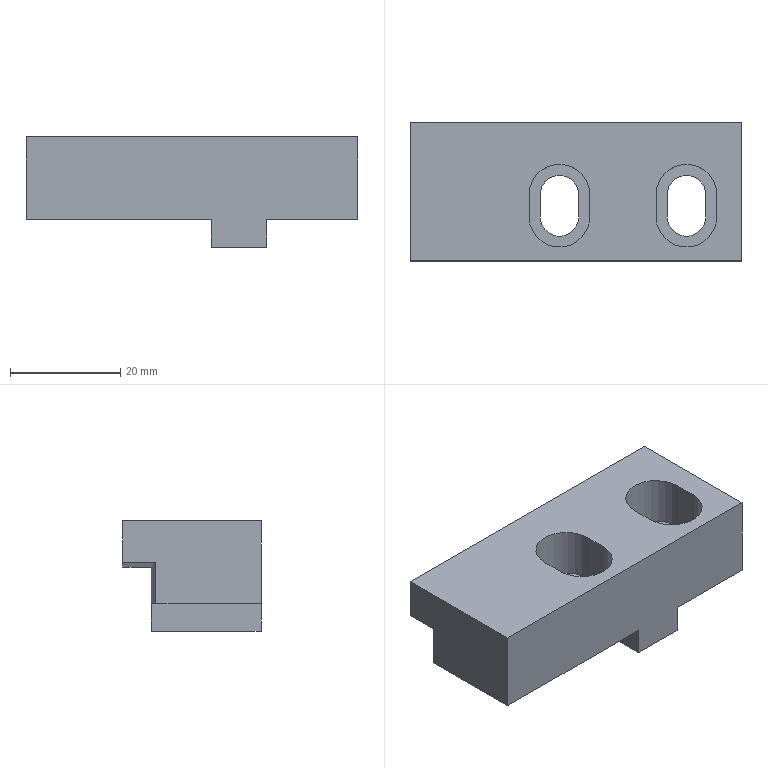Part | NX | features 1605340631 2 | 1 solid | 34 faces | box 60 x 25 x 20 mm | volume 18121 mm3 | plane 26 | cylinder 8 | commonest cylinder face diameters 7 x4 11 x4
STEP:
#1=CARTESIAN_POINT('',(576.,-115.2,-1.5));
#2=VERTEX_POINT('',#1);
#3=CARTESIAN_POINT('',(576.,-95.3,-1.5));
#4=VERTEX_POINT('',#3);
#5=CARTESIAN_POINT('',(576.,-50.,-1.5));
#6=DIRECTION('',(0.,-1.,0.));
#7=VECTOR('',#6,1000.);
#8=LINE('',#5,#7);
#9=EDGE_CURVE('',#2,#4,#8,.F.);
#10=ORIENTED_EDGE('',*,*,#9,.T.);
#11=CARTESIAN_POINT('',(587.5,-95.3,-1.5));
#12=VERTEX_POINT('',#11);
#13=CARTESIAN_POINT('',(560.128,-95.3,-1.5));
#14=DIRECTION('',(-1.,0.,0.));
#15=VECTOR('',#14,1000.);
#16=LINE('',#13,#15);
#17=EDGE_CURVE('',#12,#4,#16,.T.);
#18=ORIENTED_EDGE('',*,*,#17,.F.);
#19=CARTESIAN_POINT('',(592.5,-96.182,-1.5));
#20=VERTEX_POINT('',#19);
#21=CARTESIAN_POINT('',(592.5,-96.182,-1.5));
#22=DIRECTION('',(0.9848,-0.1736,0.));
#23=VECTOR('',#22,1000.);
#24=LINE('',#21,#23);
#25=EDGE_CURVE('',#20,#12,#24,.F.);
#26=ORIENTED_EDGE('',*,*,#25,.F.);
#27=CARTESIAN_POINT('',(592.5,-115.2,-1.5));
#28=VERTEX_POINT('',#27);
#29=CARTESIAN_POINT('',(592.5,-90.2,-1.5));
#30=DIRECTION('',(0.,1.,0.));
#31=VECTOR('',#30,1000.);
#32=LINE('',#29,#31);
#33=EDGE_CURVE('',#28,#20,#32,.T.);
#34=ORIENTED_EDGE('',*,*,#33,.F.);
#35=CARTESIAN_POINT('',(572.,-115.2,-1.5));
#36=DIRECTION('',(1.,0.,0.));
#37=VECTOR('',#36,1000.);
#38=LINE('',#35,#37);
#39=EDGE_CURVE('',#2,#28,#38,.T.);
#40=ORIENTED_EDGE('',*,*,#39,.F.);
#41=EDGE_LOOP('',(#10,#18,#26,#34,#40));
#42=FACE_BOUND('',#41,.T.);
#43=CARTESIAN_POINT('',(579.,-103.2,-1.5));
#44=VERTEX_POINT('',#43);
#45=CARTESIAN_POINT('',(586.,-103.2,-1.5));
#46=VERTEX_POINT('',#45);
#47=CARTESIAN_POINT('',(582.5,-103.2,-1.5));
#48=DIRECTION('',(0.,0.,-1.));
#49=DIRECTION('',(-1.,0.,0.));
#50=AXIS2_PLACEMENT_3D('',#47,#48,#49);
#51=CIRCLE('',#50,3.5);
#52=EDGE_CURVE('',#44,#46,#51,.T.);
#53=ORIENTED_EDGE('',*,*,#52,.F.);
#54=CARTESIAN_POINT('',(579.,-107.2,-1.5));
#55=VERTEX_POINT('',#54);
#56=CARTESIAN_POINT('',(579.,-50.,-1.5));
#57=DIRECTION('',(0.,1.,0.));
#58=VECTOR('',#57,1000.);
#59=LINE('',#56,#58);
#60=EDGE_CURVE('',#44,#55,#59,.F.);
#61=ORIENTED_EDGE('',*,*,#60,.T.);
#62=CARTESIAN_POINT('',(586.,-107.2,-1.5));
#63=VERTEX_POINT('',#62);
#64=CARTESIAN_POINT('',(582.5,-107.2,-1.5));
#65=DIRECTION('',(0.,0.,-1.));
#66=DIRECTION('',(-1.,0.,0.));
#67=AXIS2_PLACEMENT_3D('',#64,#65,#66);
#68=CIRCLE('',#67,3.5);
#69=EDGE_CURVE('',#63,#55,#68,.T.);
#70=ORIENTED_EDGE('',*,*,#69,.F.);
#71=CARTESIAN_POINT('',(586.,-50.,-1.5));
#72=DIRECTION('',(0.,-1.,0.));
#73=VECTOR('',#72,1000.);
#74=LINE('',#71,#73);
#75=EDGE_CURVE('',#63,#46,#74,.F.);
#76=ORIENTED_EDGE('',*,*,#75,.T.);
#77=EDGE_LOOP('',(#53,#61,#70,#76));
#78=FACE_BOUND('',#77,.T.);
#79=CARTESIAN_POINT('',(562.5,-50.,-1.5));
#80=DIRECTION('',(0.,0.,-1.));
#81=DIRECTION('',(-1.,0.,0.));
#82=AXIS2_PLACEMENT_3D('',#79,#80,#81);
#83=PLANE('',#82);
#84=ADVANCED_FACE('',(#42,#78),#83,.T.);
#85=ORIENTED_EDGE('',*,*,#75,.F.);
#86=CARTESIAN_POINT('',(586.,-107.2,4.5));
#87=VERTEX_POINT('',#86);
#88=CARTESIAN_POINT('',(586.,-107.2,1.5));
#89=DIRECTION('',(0.,0.,-1.));
#90=VECTOR('',#89,1000.);
#91=LINE('',#88,#90);
#92=EDGE_CURVE('',#87,#63,#91,.T.);
#93=ORIENTED_EDGE('',*,*,#92,.F.);
#94=CARTESIAN_POINT('',(586.,-103.2,4.5));
#95=VERTEX_POINT('',#94);
#96=CARTESIAN_POINT('',(586.,-105.782,4.5));
#97=DIRECTION('',(0.,-1.,0.));
#98=VECTOR('',#97,1000.);
#99=LINE('',#96,#98);
#100=EDGE_CURVE('',#95,#87,#99,.T.);
#101=ORIENTED_EDGE('',*,*,#100,.F.);
#102=CARTESIAN_POINT('',(586.,-103.2,1.5));
#103=DIRECTION('',(0.,0.,-1.));
#104=VECTOR('',#103,1000.);
#105=LINE('',#102,#104);
#106=EDGE_CURVE('',#46,#95,#105,.F.);
#107=ORIENTED_EDGE('',*,*,#106,.F.);
#108=EDGE_LOOP('',(#85,#93,#101,#107));
#109=FACE_BOUND('',#108,.T.);
#110=CARTESIAN_POINT('',(586.,-105.782,13.5));
#111=DIRECTION('',(1.,0.,0.));
#112=DIRECTION('',(0.,0.,1.));
#113=AXIS2_PLACEMENT_3D('',#110,#111,#112);
#114=PLANE('',#113);
#115=ADVANCED_FACE('',(#109),#114,.F.);
#116=CARTESIAN_POINT('',(588.,-103.2,13.5));
#117=VERTEX_POINT('',#116);
#118=CARTESIAN_POINT('',(577.,-103.2,13.5));
#119=VERTEX_POINT('',#118);
#120=CARTESIAN_POINT('',(582.5,-103.2,13.5));
#121=DIRECTION('',(0.,0.,1.));
#122=DIRECTION('',(1.,0.,0.));
#123=AXIS2_PLACEMENT_3D('',#120,#121,#122);
#124=CIRCLE('',#123,5.5);
#125=EDGE_CURVE('',#117,#119,#124,.T.);
#126=ORIENTED_EDGE('',*,*,#125,.T.);
#127=CARTESIAN_POINT('',(577.,-103.2,4.5));
#128=VERTEX_POINT('',#127);
#129=CARTESIAN_POINT('',(577.,-103.2,9.));
#130=DIRECTION('',(0.,0.,-1.));
#131=VECTOR('',#130,1000.);
#132=LINE('',#129,#131);
#133=EDGE_CURVE('',#119,#128,#132,.T.);
#134=ORIENTED_EDGE('',*,*,#133,.T.);
#135=CARTESIAN_POINT('',(588.,-103.2,4.5));
#136=VERTEX_POINT('',#135);
#137=CARTESIAN_POINT('',(582.5,-103.2,4.5));
#138=DIRECTION('',(0.,0.,-1.));
#139=DIRECTION('',(-1.,0.,0.));
#140=AXIS2_PLACEMENT_3D('',#137,#138,#139);
#141=CIRCLE('',#140,5.5);
#142=EDGE_CURVE('',#136,#128,#141,.F.);
#143=ORIENTED_EDGE('',*,*,#142,.F.);
#144=CARTESIAN_POINT('',(588.,-103.2,9.));
#145=DIRECTION('',(0.,0.,-1.));
#146=VECTOR('',#145,1000.);
#147=LINE('',#144,#146);
#148=EDGE_CURVE('',#136,#117,#147,.F.);
#149=ORIENTED_EDGE('',*,*,#148,.T.);
#150=EDGE_LOOP('',(#126,#134,#143,#149));
#151=FACE_BOUND('',#150,.T.);
#152=CARTESIAN_POINT('',(582.5,-103.2,13.5));
#153=DIRECTION('',(0.,0.,-1.));
#154=DIRECTION('',(-1.,0.,0.));
#155=AXIS2_PLACEMENT_3D('',#152,#153,#154);
#156=CYLINDRICAL_SURFACE('',#155,5.5);
#157=ADVANCED_FACE('',(#151),#156,.F.);
#158=CARTESIAN_POINT('',(588.,-107.2,4.5));
#159=VERTEX_POINT('',#158);
#160=CARTESIAN_POINT('',(577.,-107.2,4.5));
#161=VERTEX_POINT('',#160);
#162=CARTESIAN_POINT('',(582.5,-107.2,4.5));
#163=DIRECTION('',(0.,0.,-1.));
#164=DIRECTION('',(-1.,0.,0.));
#165=AXIS2_PLACEMENT_3D('',#162,#163,#164);
#166=CIRCLE('',#165,5.5);
#167=EDGE_CURVE('',#159,#161,#166,.T.);
#168=ORIENTED_EDGE('',*,*,#167,.T.);
#169=CARTESIAN_POINT('',(577.,-107.2,13.5));
#170=VERTEX_POINT('',#169);
#171=CARTESIAN_POINT('',(577.,-107.2,9.));
#172=DIRECTION('',(0.,0.,-1.));
#173=VECTOR('',#172,1000.);
#174=LINE('',#171,#173);
#175=EDGE_CURVE('',#161,#170,#174,.F.);
#176=ORIENTED_EDGE('',*,*,#175,.T.);
#177=CARTESIAN_POINT('',(588.,-107.2,13.5));
#178=VERTEX_POINT('',#177);
#179=CARTESIAN_POINT('',(582.5,-107.2,13.5));
#180=DIRECTION('',(0.,0.,1.));
#181=DIRECTION('',(1.,0.,0.));
#182=AXIS2_PLACEMENT_3D('',#179,#180,#181);
#183=CIRCLE('',#182,5.5);
#184=EDGE_CURVE('',#170,#178,#183,.T.);
#185=ORIENTED_EDGE('',*,*,#184,.T.);
#186=CARTESIAN_POINT('',(588.,-107.2,9.));
#187=DIRECTION('',(0.,0.,-1.));
#188=VECTOR('',#187,1000.);
#189=LINE('',#186,#188);
#190=EDGE_CURVE('',#178,#159,#189,.T.);
#191=ORIENTED_EDGE('',*,*,#190,.T.);
#192=EDGE_LOOP('',(#168,#176,#185,#191));
#193=FACE_BOUND('',#192,.T.);
#194=CARTESIAN_POINT('',(582.5,-107.2,13.5));
#195=DIRECTION('',(0.,0.,-1.));
#196=DIRECTION('',(-1.,0.,0.));
#197=AXIS2_PLACEMENT_3D('',#194,#195,#196);
#198=CYLINDRICAL_SURFACE('',#197,5.5);
#199=ADVANCED_FACE('',(#193),#198,.F.);
#200=CARTESIAN_POINT('',(579.,-107.2,4.5));
#201=VERTEX_POINT('',#200);
#202=CARTESIAN_POINT('',(582.5,-107.2,4.5));
#203=DIRECTION('',(0.,0.,1.));
#204=DIRECTION('',(1.,0.,0.));
#205=AXIS2_PLACEMENT_3D('',#202,#203,#204);
#206=CIRCLE('',#205,3.5);
#207=EDGE_CURVE('',#87,#201,#206,.F.);
#208=ORIENTED_EDGE('',*,*,#207,.T.);
#209=CARTESIAN_POINT('',(579.,-103.2,4.5));
#210=VERTEX_POINT('',#209);
#211=CARTESIAN_POINT('',(579.,-105.782,4.5));
#212=DIRECTION('',(0.,1.,0.));
#213=VECTOR('',#212,1000.);
#214=LINE('',#211,#213);
#215=EDGE_CURVE('',#201,#210,#214,.T.);
#216=ORIENTED_EDGE('',*,*,#215,.T.);
#217=CARTESIAN_POINT('',(582.5,-103.2,4.5));
#218=DIRECTION('',(0.,0.,1.));
#219=DIRECTION('',(1.,0.,0.));
#220=AXIS2_PLACEMENT_3D('',#217,#218,#219);
#221=CIRCLE('',#220,3.5);
#222=EDGE_CURVE('',#95,#210,#221,.T.);
#223=ORIENTED_EDGE('',*,*,#222,.F.);
#224=ORIENTED_EDGE('',*,*,#100,.T.);
#225=EDGE_LOOP('',(#208,#216,#223,#224));
#226=FACE_BOUND('',#225,.T.);
#227=ORIENTED_EDGE('',*,*,#167,.F.);
#228=CARTESIAN_POINT('',(588.,-107.2,4.5));
#229=DIRECTION('',(0.,1.,0.));
#230=VECTOR('',#229,1000.);
#231=LINE('',#228,#230);
#232=EDGE_CURVE('',#159,#136,#231,.T.);
#233=ORIENTED_EDGE('',*,*,#232,.T.);
#234=ORIENTED_EDGE('',*,*,#142,.T.);
#235=CARTESIAN_POINT('',(577.,-107.2,4.5));
#236=DIRECTION('',(0.,-1.,0.));
#237=VECTOR('',#236,1000.);
#238=LINE('',#235,#237);
#239=EDGE_CURVE('',#128,#161,#238,.T.);
#240=ORIENTED_EDGE('',*,*,#239,.T.);
#241=EDGE_LOOP('',(#227,#233,#234,#240));
#242=FACE_BOUND('',#241,.T.);
#243=CARTESIAN_POINT('',(582.5,-107.2,4.5));
#244=DIRECTION('',(0.,0.,-1.));
#245=DIRECTION('',(1.,0.,0.));
#246=AXIS2_PLACEMENT_3D('',#243,#244,#245);
#247=PLANE('',#246);
#248=ADVANCED_FACE('',(#226,#242),#247,.F.);
#249=ORIENTED_EDGE('',*,*,#232,.F.);
#250=ORIENTED_EDGE('',*,*,#190,.F.);
#251=CARTESIAN_POINT('',(588.,-107.951,13.5));
#252=DIRECTION('',(0.,1.,0.));
#253=VECTOR('',#252,1000.);
#254=LINE('',#251,#253);
#255=EDGE_CURVE('',#117,#178,#254,.F.);
#256=ORIENTED_EDGE('',*,*,#255,.F.);
#257=ORIENTED_EDGE('',*,*,#148,.F.);
#258=EDGE_LOOP('',(#249,#250,#256,#257));
#259=FACE_BOUND('',#258,.T.);
#260=CARTESIAN_POINT('',(588.,-105.836,13.5));
#261=DIRECTION('',(1.,0.,0.));
#262=DIRECTION('',(0.,0.,1.));
#263=AXIS2_PLACEMENT_3D('',#260,#261,#262);
#264=PLANE('',#263);
#265=ADVANCED_FACE('',(#259),#264,.F.);
#266=CARTESIAN_POINT('',(577.,-107.951,13.5));
#267=DIRECTION('',(0.,-1.,0.));
#268=VECTOR('',#267,1000.);
#269=LINE('',#266,#268);
#270=EDGE_CURVE('',#170,#119,#269,.F.);
#271=ORIENTED_EDGE('',*,*,#270,.F.);
#272=ORIENTED_EDGE('',*,*,#175,.F.);
#273=ORIENTED_EDGE('',*,*,#239,.F.);
#274=ORIENTED_EDGE('',*,*,#133,.F.);
#275=EDGE_LOOP('',(#271,#272,#273,#274));
#276=FACE_BOUND('',#275,.T.);
#277=CARTESIAN_POINT('',(577.,-105.836,13.5));
#278=DIRECTION('',(-1.,0.,0.));
#279=DIRECTION('',(0.,0.,-1.));
#280=AXIS2_PLACEMENT_3D('',#277,#278,#279);
#281=PLANE('',#280);
#282=ADVANCED_FACE('',(#276),#281,.F.);
#283=ORIENTED_EDGE('',*,*,#215,.F.);
#284=CARTESIAN_POINT('',(579.,-107.2,1.5));
#285=DIRECTION('',(0.,0.,-1.));
#286=VECTOR('',#285,1000.);
#287=LINE('',#284,#286);
#288=EDGE_CURVE('',#55,#201,#287,.F.);
#289=ORIENTED_EDGE('',*,*,#288,.F.);
#290=ORIENTED_EDGE('',*,*,#60,.F.);
#291=CARTESIAN_POINT('',(579.,-103.2,1.5));
#292=DIRECTION('',(0.,0.,-1.));
#293=VECTOR('',#292,1000.);
#294=LINE('',#291,#293);
#295=EDGE_CURVE('',#210,#44,#294,.T.);
#296=ORIENTED_EDGE('',*,*,#295,.F.);
#297=EDGE_LOOP('',(#283,#289,#290,#296));
#298=FACE_BOUND('',#297,.T.);
#299=CARTESIAN_POINT('',(579.,-105.782,13.5));
#300=DIRECTION('',(-1.,0.,0.));
#301=DIRECTION('',(0.,0.,-1.));
#302=AXIS2_PLACEMENT_3D('',#299,#300,#301);
#303=PLANE('',#302);
#304=ADVANCED_FACE('',(#298),#303,.F.);
#305=ORIENTED_EDGE('',*,*,#69,.T.);
#306=ORIENTED_EDGE('',*,*,#288,.T.);
#307=ORIENTED_EDGE('',*,*,#207,.F.);
#308=ORIENTED_EDGE('',*,*,#92,.T.);
#309=EDGE_LOOP('',(#305,#306,#307,#308));
#310=FACE_BOUND('',#309,.T.);
#311=CARTESIAN_POINT('',(582.5,-107.2,13.5));
#312=DIRECTION('',(0.,0.,-1.));
#313=DIRECTION('',(-1.,0.,0.));
#314=AXIS2_PLACEMENT_3D('',#311,#312,#313);
#315=CYLINDRICAL_SURFACE('',#314,3.5);
#316=ADVANCED_FACE('',(#310),#315,.F.);
#317=ORIENTED_EDGE('',*,*,#222,.T.);
#318=ORIENTED_EDGE('',*,*,#295,.T.);
#319=ORIENTED_EDGE('',*,*,#52,.T.);
#320=ORIENTED_EDGE('',*,*,#106,.T.);
#321=EDGE_LOOP('',(#317,#318,#319,#320));
#322=FACE_BOUND('',#321,.T.);
#323=CARTESIAN_POINT('',(582.5,-103.2,13.5));
#324=DIRECTION('',(0.,0.,-1.));
#325=DIRECTION('',(-1.,0.,0.));
#326=AXIS2_PLACEMENT_3D('',#323,#324,#325);
#327=CYLINDRICAL_SURFACE('',#326,3.5);
#328=ADVANCED_FACE('',(#322),#327,.F.);
#329=CARTESIAN_POINT('',(563.,-107.2,4.5));
#330=VERTEX_POINT('',#329);
#331=CARTESIAN_POINT('',(556.,-107.2,4.5));
#332=VERTEX_POINT('',#331);
#333=CARTESIAN_POINT('',(559.5,-107.2,4.5));
#334=DIRECTION('',(0.,0.,-1.));
#335=DIRECTION('',(-1.,0.,0.));
#336=AXIS2_PLACEMENT_3D('',#333,#334,#335);
#337=CIRCLE('',#336,3.5);
#338=EDGE_CURVE('',#330,#332,#337,.T.);
#339=ORIENTED_EDGE('',*,*,#338,.T.);
#340=CARTESIAN_POINT('',(556.,-103.2,4.5));
#341=VERTEX_POINT('',#340);
#342=CARTESIAN_POINT('',(556.,-105.782,4.5));
#343=DIRECTION('',(0.,-1.,0.));
#344=VECTOR('',#343,1000.);
#345=LINE('',#342,#344);
#346=EDGE_CURVE('',#332,#341,#345,.F.);
#347=ORIENTED_EDGE('',*,*,#346,.T.);
#348=CARTESIAN_POINT('',(563.,-103.2,4.5));
#349=VERTEX_POINT('',#348);
#350=CARTESIAN_POINT('',(559.5,-103.2,4.5));
#351=DIRECTION('',(0.,0.,-1.));
#352=DIRECTION('',(-1.,0.,0.));
#353=AXIS2_PLACEMENT_3D('',#350,#351,#352);
#354=CIRCLE('',#353,3.5);
#355=EDGE_CURVE('',#349,#341,#354,.F.);
#356=ORIENTED_EDGE('',*,*,#355,.F.);
#357=CARTESIAN_POINT('',(563.,-105.782,4.5));
#358=DIRECTION('',(0.,1.,0.));
#359=VECTOR('',#358,1000.);
#360=LINE('',#357,#359);
#361=EDGE_CURVE('',#349,#330,#360,.F.);
#362=ORIENTED_EDGE('',*,*,#361,.T.);
#363=EDGE_LOOP('',(#339,#347,#356,#362));
#364=FACE_BOUND('',#363,.T.);
#365=CARTESIAN_POINT('',(565.,-107.2,4.5));
#366=VERTEX_POINT('',#365);
#367=CARTESIAN_POINT('',(554.,-107.2,4.5));
#368=VERTEX_POINT('',#367);
#369=CARTESIAN_POINT('',(559.5,-107.2,4.5));
#370=DIRECTION('',(0.,0.,1.));
#371=DIRECTION('',(1.,0.,0.));
#372=AXIS2_PLACEMENT_3D('',#369,#370,#371);
#373=CIRCLE('',#372,5.5);
#374=EDGE_CURVE('',#366,#368,#373,.F.);
#375=ORIENTED_EDGE('',*,*,#374,.F.);
#376=CARTESIAN_POINT('',(565.,-103.2,4.5));
#377=VERTEX_POINT('',#376);
#378=CARTESIAN_POINT('',(565.,-107.2,4.5));
#379=DIRECTION('',(0.,-1.,0.));
#380=VECTOR('',#379,1000.);
#381=LINE('',#378,#380);
#382=EDGE_CURVE('',#366,#377,#381,.F.);
#383=ORIENTED_EDGE('',*,*,#382,.T.);
#384=CARTESIAN_POINT('',(554.,-103.2,4.5));
#385=VERTEX_POINT('',#384);
#386=CARTESIAN_POINT('',(559.5,-103.2,4.5));
#387=DIRECTION('',(0.,0.,1.));
#388=DIRECTION('',(1.,0.,0.));
#389=AXIS2_PLACEMENT_3D('',#386,#387,#388);
#390=CIRCLE('',#389,5.5);
#391=EDGE_CURVE('',#377,#385,#390,.T.);
#392=ORIENTED_EDGE('',*,*,#391,.T.);
#393=CARTESIAN_POINT('',(554.,-107.2,4.5));
#394=DIRECTION('',(0.,1.,0.));
#395=VECTOR('',#394,1000.);
#396=LINE('',#393,#395);
#397=EDGE_CURVE('',#385,#368,#396,.F.);
#398=ORIENTED_EDGE('',*,*,#397,.T.);
#399=EDGE_LOOP('',(#375,#383,#392,#398));
#400=FACE_BOUND('',#399,.T.);
#401=CARTESIAN_POINT('',(542.5,-107.2,4.5));
#402=DIRECTION('',(0.,0.,-1.));
#403=DIRECTION('',(-1.,0.,0.));
#404=AXIS2_PLACEMENT_3D('',#401,#402,#403);
#405=PLANE('',#404);
#406=ADVANCED_FACE('',(#364,#400),#405,.F.);
#407=CARTESIAN_POINT('',(537.5,-95.3,5.1));
#408=VERTEX_POINT('',#407);
#409=CARTESIAN_POINT('',(532.5,-96.182,5.982));
#410=VERTEX_POINT('',#409);
#411=CARTESIAN_POINT('',(535.027,-95.736,5.536));
#412=DIRECTION('',(-0.9703,-0.1711,0.1711));
#413=VECTOR('',#412,1000.);
#414=LINE('',#411,#413);
#415=EDGE_CURVE('',#408,#410,#414,.T.);
#416=ORIENTED_EDGE('',*,*,#415,.T.);
#417=CARTESIAN_POINT('',(532.5,-90.2,5.982));
#418=VERTEX_POINT('',#417);
#419=CARTESIAN_POINT('',(532.5,-95.3,5.982));
#420=DIRECTION('',(0.,-1.,0.));
#421=VECTOR('',#420,1000.);
#422=LINE('',#419,#421);
#423=EDGE_CURVE('',#418,#410,#422,.T.);
#424=ORIENTED_EDGE('',*,*,#423,.F.);
#425=CARTESIAN_POINT('',(537.5,-90.2,5.1));
#426=VERTEX_POINT('',#425);
#427=CARTESIAN_POINT('',(543.856,-90.2,3.979));
#428=DIRECTION('',(-0.9848,0.,0.1736));
#429=VECTOR('',#428,1000.);
#430=LINE('',#427,#429);
#431=EDGE_CURVE('',#426,#418,#430,.T.);
#432=ORIENTED_EDGE('',*,*,#431,.F.);
#433=CARTESIAN_POINT('',(537.5,-92.2,5.1));
#434=DIRECTION('',(0.,1.,0.));
#435=VECTOR('',#434,1000.);
#436=LINE('',#433,#435);
#437=EDGE_CURVE('',#408,#426,#436,.T.);
#438=ORIENTED_EDGE('',*,*,#437,.F.);
#439=EDGE_LOOP('',(#416,#424,#432,#438));
#440=FACE_BOUND('',#439,.T.);
#441=CARTESIAN_POINT('',(537.5,-110.2,5.1));
#442=DIRECTION('',(-0.1736,0.,-0.9848));
#443=DIRECTION('',(0.,-1.,0.));
#444=AXIS2_PLACEMENT_3D('',#441,#442,#443);
#445=PLANE('',#444);
#446=ADVANCED_FACE('',(#440),#445,.T.);
#447=CARTESIAN_POINT('',(587.5,-90.2,5.1));
#448=VERTEX_POINT('',#447);
#449=CARTESIAN_POINT('',(552.,-90.2,5.1));
#450=DIRECTION('',(1.,0.,0.));
#451=VECTOR('',#450,1000.);
#452=LINE('',#449,#451);
#453=EDGE_CURVE('',#426,#448,#452,.T.);
#454=ORIENTED_EDGE('',*,*,#453,.T.);
#455=CARTESIAN_POINT('',(587.5,-95.3,5.1));
#456=VERTEX_POINT('',#455);
#457=CARTESIAN_POINT('',(587.5,-95.3,5.1));
#458=DIRECTION('',(0.,-1.,0.));
#459=VECTOR('',#458,1000.);
#460=LINE('',#457,#459);
#461=EDGE_CURVE('',#448,#456,#460,.T.);
#462=ORIENTED_EDGE('',*,*,#461,.T.);
#463=CARTESIAN_POINT('',(560.128,-95.3,5.1));
#464=DIRECTION('',(1.,0.,0.));
#465=VECTOR('',#464,1000.);
#466=LINE('',#463,#465);
#467=EDGE_CURVE('',#408,#456,#466,.T.);
#468=ORIENTED_EDGE('',*,*,#467,.F.);
#469=ORIENTED_EDGE('',*,*,#437,.T.);
#470=EDGE_LOOP('',(#454,#462,#468,#469));
#471=FACE_BOUND('',#470,.T.);
#472=CARTESIAN_POINT('',(552.,-110.2,5.1));
#473=DIRECTION('',(0.,0.,1.));
#474=DIRECTION('',(1.,0.,0.));
#475=AXIS2_PLACEMENT_3D('',#472,#473,#474);
#476=PLANE('',#475);
#477=ADVANCED_FACE('',(#471),#476,.F.);
#478=CARTESIAN_POINT('',(592.5,-90.2,5.982));
#479=VERTEX_POINT('',#478);
#480=CARTESIAN_POINT('',(561.747,-90.2,0.5591));
#481=DIRECTION('',(-0.9848,0.,-0.1736));
#482=VECTOR('',#481,1000.);
#483=LINE('',#480,#482);
#484=EDGE_CURVE('',#479,#448,#483,.T.);
#485=ORIENTED_EDGE('',*,*,#484,.F.);
#486=CARTESIAN_POINT('',(592.5,-96.182,5.982));
#487=VERTEX_POINT('',#486);
#488=CARTESIAN_POINT('',(592.5,-92.2,5.982));
#489=DIRECTION('',(0.,1.,0.));
#490=VECTOR('',#489,1000.);
#491=LINE('',#488,#490);
#492=EDGE_CURVE('',#487,#479,#491,.T.);
#493=ORIENTED_EDGE('',*,*,#492,.F.);
#494=CARTESIAN_POINT('',(589.973,-95.736,5.536));
#495=DIRECTION('',(-0.9703,0.1711,-0.1711));
#496=VECTOR('',#495,1000.);
#497=LINE('',#494,#496);
#498=EDGE_CURVE('',#487,#456,#497,.T.);
#499=ORIENTED_EDGE('',*,*,#498,.T.);
#500=ORIENTED_EDGE('',*,*,#461,.F.);
#501=EDGE_LOOP('',(#485,#493,#499,#500));
#502=FACE_BOUND('',#501,.T.);
#503=CARTESIAN_POINT('',(587.5,-110.2,5.1));
#504=DIRECTION('',(0.1736,0.,-0.9848));
#505=DIRECTION('',(0.,1.,0.));
#506=AXIS2_PLACEMENT_3D('',#503,#504,#505);
#507=PLANE('',#506);
#508=ADVANCED_FACE('',(#502),#507,.T.);
#509=CARTESIAN_POINT('',(592.5,-96.182,-36.501));
#510=DIRECTION('',(0.,0.,1.));
#511=VECTOR('',#510,1000.);
#512=LINE('',#509,#511);
#513=EDGE_CURVE('',#20,#487,#512,.T.);
#514=ORIENTED_EDGE('',*,*,#513,.F.);
#515=ORIENTED_EDGE('',*,*,#25,.T.);
#516=CARTESIAN_POINT('',(587.5,-95.3,-0.1));
#517=DIRECTION('',(0.,0.,-1.));
#518=VECTOR('',#517,1000.);
#519=LINE('',#516,#518);
#520=EDGE_CURVE('',#456,#12,#519,.T.);
#521=ORIENTED_EDGE('',*,*,#520,.F.);
#522=ORIENTED_EDGE('',*,*,#498,.F.);
#523=EDGE_LOOP('',(#514,#515,#521,#522));
#524=FACE_BOUND('',#523,.T.);
#525=CARTESIAN_POINT('',(592.5,-96.182,-36.501));
#526=DIRECTION('',(-0.1736,-0.9848,0.));
#527=DIRECTION('',(0.,0.,1.));
#528=AXIS2_PLACEMENT_3D('',#525,#526,#527);
#529=PLANE('',#528);
#530=ADVANCED_FACE('',(#524),#529,.F.);
#531=ORIENTED_EDGE('',*,*,#17,.T.);
#532=CARTESIAN_POINT('',(576.,-95.3,-6.5));
#533=VERTEX_POINT('',#532);
#534=CARTESIAN_POINT('',(576.,-95.3,-6.5));
#535=DIRECTION('',(0.,0.,1.));
#536=VECTOR('',#535,1000.);
#537=LINE('',#534,#536);
#538=EDGE_CURVE('',#4,#533,#537,.F.);
#539=ORIENTED_EDGE('',*,*,#538,.T.);
#540=CARTESIAN_POINT('',(566.,-95.3,-6.5));
#541=VERTEX_POINT('',#540);
#542=CARTESIAN_POINT('',(560.128,-95.3,-6.5));
#543=DIRECTION('',(-1.,0.,0.));
#544=VECTOR('',#543,1000.);
#545=LINE('',#542,#544);
#546=EDGE_CURVE('',#541,#533,#545,.F.);
#547=ORIENTED_EDGE('',*,*,#546,.F.);
#548=CARTESIAN_POINT('',(566.,-95.3,-1.5));
#549=VERTEX_POINT('',#548);
#550=CARTESIAN_POINT('',(566.,-95.3,-0.1));
#551=DIRECTION('',(0.,0.,1.));
#552=VECTOR('',#551,1000.);
#553=LINE('',#550,#552);
#554=EDGE_CURVE('',#549,#541,#553,.F.);
#555=ORIENTED_EDGE('',*,*,#554,.F.);
#556=CARTESIAN_POINT('',(537.5,-95.3,-1.5));
#557=VERTEX_POINT('',#556);
#558=CARTESIAN_POINT('',(560.128,-95.3,-1.5));
#559=DIRECTION('',(-1.,0.,0.));
#560=VECTOR('',#559,1000.);
#561=LINE('',#558,#560);
#562=EDGE_CURVE('',#549,#557,#561,.T.);
#563=ORIENTED_EDGE('',*,*,#562,.T.);
#564=CARTESIAN_POINT('',(537.5,-95.3,-0.1));
#565=DIRECTION('',(0.,0.,1.));
#566=VECTOR('',#565,1000.);
#567=LINE('',#564,#566);
#568=EDGE_CURVE('',#557,#408,#567,.T.);
#569=ORIENTED_EDGE('',*,*,#568,.T.);
#570=ORIENTED_EDGE('',*,*,#467,.T.);
#571=ORIENTED_EDGE('',*,*,#520,.T.);
#572=EDGE_LOOP('',(#531,#539,#547,#555,#563,#569,#570,#571));
#573=FACE_BOUND('',#572,.T.);
#574=CARTESIAN_POINT('',(560.128,-95.3,-0.1));
#575=DIRECTION('',(0.,1.,0.));
#576=DIRECTION('',(-1.,0.,0.));
#577=AXIS2_PLACEMENT_3D('',#574,#575,#576);
#578=PLANE('',#577);
#579=ADVANCED_FACE('',(#573),#578,.T.);
#580=ORIENTED_EDGE('',*,*,#568,.F.);
#581=CARTESIAN_POINT('',(532.5,-96.182,-1.5));
#582=VERTEX_POINT('',#581);
#583=CARTESIAN_POINT('',(532.5,-96.182,-1.5));
#584=DIRECTION('',(0.9848,0.1736,0.));
#585=VECTOR('',#584,1000.);
#586=LINE('',#583,#585);
#587=EDGE_CURVE('',#557,#582,#586,.F.);
#588=ORIENTED_EDGE('',*,*,#587,.T.);
#589=CARTESIAN_POINT('',(532.5,-96.182,-36.501));
#590=DIRECTION('',(0.,0.,-1.));
#591=VECTOR('',#590,1000.);
#592=LINE('',#589,#591);
#593=EDGE_CURVE('',#410,#582,#592,.T.);
#594=ORIENTED_EDGE('',*,*,#593,.F.);
#595=ORIENTED_EDGE('',*,*,#415,.F.);
#596=EDGE_LOOP('',(#580,#588,#594,#595));
#597=FACE_BOUND('',#596,.T.);
#598=CARTESIAN_POINT('',(532.5,-96.182,-36.501));
#599=DIRECTION('',(0.1736,-0.9848,0.));
#600=DIRECTION('',(0.,0.,-1.));
#601=AXIS2_PLACEMENT_3D('',#598,#599,#600);
#602=PLANE('',#601);
#603=ADVANCED_FACE('',(#597),#602,.F.);
#604=CARTESIAN_POINT('',(565.,-103.2,13.5));
#605=VERTEX_POINT('',#604);
#606=CARTESIAN_POINT('',(565.,-107.2,13.5));
#607=VERTEX_POINT('',#606);
#608=CARTESIAN_POINT('',(565.,-107.951,13.5));
#609=DIRECTION('',(0.,1.,0.));
#610=VECTOR('',#609,1000.);
#611=LINE('',#608,#610);
#612=EDGE_CURVE('',#605,#607,#611,.F.);
#613=ORIENTED_EDGE('',*,*,#612,.F.);
#614=CARTESIAN_POINT('',(565.,-103.2,9.));
#615=DIRECTION('',(0.,0.,-1.));
#616=VECTOR('',#615,1000.);
#617=LINE('',#614,#616);
#618=EDGE_CURVE('',#377,#605,#617,.F.);
#619=ORIENTED_EDGE('',*,*,#618,.F.);
#620=ORIENTED_EDGE('',*,*,#382,.F.);
#621=CARTESIAN_POINT('',(565.,-107.2,9.));
#622=DIRECTION('',(0.,0.,-1.));
#623=VECTOR('',#622,1000.);
#624=LINE('',#621,#623);
#625=EDGE_CURVE('',#607,#366,#624,.T.);
#626=ORIENTED_EDGE('',*,*,#625,.F.);
#627=EDGE_LOOP('',(#613,#619,#620,#626));
#628=FACE_BOUND('',#627,.T.);
#629=CARTESIAN_POINT('',(565.,-105.836,13.5));
#630=DIRECTION('',(1.,0.,0.));
#631=DIRECTION('',(0.,0.,-1.));
#632=AXIS2_PLACEMENT_3D('',#629,#630,#631);
#633=PLANE('',#632);
#634=ADVANCED_FACE('',(#628),#633,.F.);
#635=CARTESIAN_POINT('',(554.,-103.2,13.5));
#636=VERTEX_POINT('',#635);
#637=CARTESIAN_POINT('',(559.5,-103.2,13.5));
#638=DIRECTION('',(0.,0.,-1.));
#639=DIRECTION('',(1.,0.,0.));
#640=AXIS2_PLACEMENT_3D('',#637,#638,#639);
#641=CIRCLE('',#640,5.5);
#642=EDGE_CURVE('',#636,#605,#641,.T.);
#643=ORIENTED_EDGE('',*,*,#642,.F.);
#644=CARTESIAN_POINT('',(554.,-103.2,9.));
#645=DIRECTION('',(0.,0.,-1.));
#646=VECTOR('',#645,1000.);
#647=LINE('',#644,#646);
#648=EDGE_CURVE('',#636,#385,#647,.T.);
#649=ORIENTED_EDGE('',*,*,#648,.T.);
#650=ORIENTED_EDGE('',*,*,#391,.F.);
#651=ORIENTED_EDGE('',*,*,#618,.T.);
#652=EDGE_LOOP('',(#643,#649,#650,#651));
#653=FACE_BOUND('',#652,.T.);
#654=CARTESIAN_POINT('',(559.5,-103.2,13.5));
#655=DIRECTION('',(0.,0.,-1.));
#656=DIRECTION('',(1.,0.,0.));
#657=AXIS2_PLACEMENT_3D('',#654,#655,#656);
#658=CYLINDRICAL_SURFACE('',#657,5.5);
#659=ADVANCED_FACE('',(#653),#658,.F.);
#660=ORIENTED_EDGE('',*,*,#397,.F.);
#661=ORIENTED_EDGE('',*,*,#648,.F.);
#662=CARTESIAN_POINT('',(554.,-107.2,13.5));
#663=VERTEX_POINT('',#662);
#664=CARTESIAN_POINT('',(554.,-107.951,13.5));
#665=DIRECTION('',(0.,-1.,0.));
#666=VECTOR('',#665,1000.);
#667=LINE('',#664,#666);
#668=EDGE_CURVE('',#663,#636,#667,.F.);
#669=ORIENTED_EDGE('',*,*,#668,.F.);
#670=CARTESIAN_POINT('',(554.,-107.2,9.));
#671=DIRECTION('',(0.,0.,-1.));
#672=VECTOR('',#671,1000.);
#673=LINE('',#670,#672);
#674=EDGE_CURVE('',#368,#663,#673,.F.);
#675=ORIENTED_EDGE('',*,*,#674,.F.);
#676=EDGE_LOOP('',(#660,#661,#669,#675));
#677=FACE_BOUND('',#676,.T.);
#678=CARTESIAN_POINT('',(554.,-105.836,13.5));
#679=DIRECTION('',(-1.,0.,0.));
#680=DIRECTION('',(0.,0.,1.));
#681=AXIS2_PLACEMENT_3D('',#678,#679,#680);
#682=PLANE('',#681);
#683=ADVANCED_FACE('',(#677),#682,.F.);
#684=ORIENTED_EDGE('',*,*,#374,.T.);
#685=ORIENTED_EDGE('',*,*,#674,.T.);
#686=CARTESIAN_POINT('',(559.5,-107.2,13.5));
#687=DIRECTION('',(0.,0.,-1.));
#688=DIRECTION('',(1.,0.,0.));
#689=AXIS2_PLACEMENT_3D('',#686,#687,#688);
#690=CIRCLE('',#689,5.5);
#691=EDGE_CURVE('',#607,#663,#690,.T.);
#692=ORIENTED_EDGE('',*,*,#691,.F.);
#693=ORIENTED_EDGE('',*,*,#625,.T.);
#694=EDGE_LOOP('',(#684,#685,#692,#693));
#695=FACE_BOUND('',#694,.T.);
#696=CARTESIAN_POINT('',(559.5,-107.2,13.5));
#697=DIRECTION('',(0.,0.,-1.));
#698=DIRECTION('',(1.,0.,0.));
#699=AXIS2_PLACEMENT_3D('',#696,#697,#698);
#700=CYLINDRICAL_SURFACE('',#699,5.5);
#701=ADVANCED_FACE('',(#695),#700,.F.);
#702=CARTESIAN_POINT('',(592.5,-115.2,13.5));
#703=VERTEX_POINT('',#702);
#704=CARTESIAN_POINT('',(592.5,-115.2,-36.501));
#705=DIRECTION('',(0.,0.,-1.));
#706=VECTOR('',#705,1000.);
#707=LINE('',#704,#706);
#708=EDGE_CURVE('',#703,#28,#707,.T.);
#709=ORIENTED_EDGE('',*,*,#708,.T.);
#710=ORIENTED_EDGE('',*,*,#33,.T.);
#711=ORIENTED_EDGE('',*,*,#513,.T.);
#712=ORIENTED_EDGE('',*,*,#492,.T.);
#713=CARTESIAN_POINT('',(592.5,-90.2,13.5));
#714=VERTEX_POINT('',#713);
#715=CARTESIAN_POINT('',(592.5,-90.2,-34.901));
#716=DIRECTION('',(0.,0.,-1.));
#717=VECTOR('',#716,1000.);
#718=LINE('',#715,#717);
#719=EDGE_CURVE('',#714,#479,#718,.T.);
#720=ORIENTED_EDGE('',*,*,#719,.F.);
#721=CARTESIAN_POINT('',(592.5,-90.2,13.5));
#722=DIRECTION('',(0.,1.,0.));
#723=VECTOR('',#722,1000.);
#724=LINE('',#721,#723);
#725=EDGE_CURVE('',#703,#714,#724,.T.);
#726=ORIENTED_EDGE('',*,*,#725,.F.);
#727=EDGE_LOOP('',(#709,#710,#711,#712,#720,#726));
#728=FACE_BOUND('',#727,.T.);
#729=CARTESIAN_POINT('',(592.5,-90.2,-36.501));
#730=DIRECTION('',(1.,0.,0.));
#731=DIRECTION('',(0.,0.,-1.));
#732=AXIS2_PLACEMENT_3D('',#729,#730,#731);
#733=PLANE('',#732);
#734=ADVANCED_FACE('',(#728),#733,.T.);
#735=CARTESIAN_POINT('',(532.5,-115.2,-1.5));
#736=VERTEX_POINT('',#735);
#737=CARTESIAN_POINT('',(566.,-115.2,-1.5));
#738=VERTEX_POINT('',#737);
#739=CARTESIAN_POINT('',(572.,-115.2,-1.5));
#740=DIRECTION('',(1.,0.,0.));
#741=VECTOR('',#740,1000.);
#742=LINE('',#739,#741);
#743=EDGE_CURVE('',#736,#738,#742,.T.);
#744=ORIENTED_EDGE('',*,*,#743,.T.);
#745=CARTESIAN_POINT('',(566.,-115.2,-6.5));
#746=VERTEX_POINT('',#745);
#747=CARTESIAN_POINT('',(566.,-115.2,-6.5));
#748=DIRECTION('',(0.,0.,1.));
#749=VECTOR('',#748,1000.);
#750=LINE('',#747,#749);
#751=EDGE_CURVE('',#738,#746,#750,.F.);
#752=ORIENTED_EDGE('',*,*,#751,.T.);
#753=CARTESIAN_POINT('',(576.,-115.2,-6.5));
#754=VERTEX_POINT('',#753);
#755=CARTESIAN_POINT('',(572.,-115.2,-6.5));
#756=DIRECTION('',(1.,0.,0.));
#757=VECTOR('',#756,1000.);
#758=LINE('',#755,#757);
#759=EDGE_CURVE('',#754,#746,#758,.F.);
#760=ORIENTED_EDGE('',*,*,#759,.F.);
#761=CARTESIAN_POINT('',(576.,-115.2,-36.501));
#762=DIRECTION('',(0.,0.,1.));
#763=VECTOR('',#762,1000.);
#764=LINE('',#761,#763);
#765=EDGE_CURVE('',#2,#754,#764,.F.);
#766=ORIENTED_EDGE('',*,*,#765,.F.);
#767=ORIENTED_EDGE('',*,*,#39,.T.);
#768=ORIENTED_EDGE('',*,*,#708,.F.);
#769=CARTESIAN_POINT('',(532.5,-115.2,13.5));
#770=VERTEX_POINT('',#769);
#771=CARTESIAN_POINT('',(572.,-115.2,13.5));
#772=DIRECTION('',(1.,0.,0.));
#773=VECTOR('',#772,1000.);
#774=LINE('',#771,#773);
#775=EDGE_CURVE('',#770,#703,#774,.T.);
#776=ORIENTED_EDGE('',*,*,#775,.F.);
#777=CARTESIAN_POINT('',(532.5,-115.2,-36.501));
#778=DIRECTION('',(0.,0.,-1.));
#779=VECTOR('',#778,1000.);
#780=LINE('',#777,#779);
#781=EDGE_CURVE('',#770,#736,#780,.T.);
#782=ORIENTED_EDGE('',*,*,#781,.T.);
#783=EDGE_LOOP('',(#744,#752,#760,#766,#767,#768,#776,#782));
#784=FACE_BOUND('',#783,.T.);
#785=CARTESIAN_POINT('',(572.,-115.2,-36.501));
#786=DIRECTION('',(0.,-1.,0.));
#787=DIRECTION('',(0.,0.,-1.));
#788=AXIS2_PLACEMENT_3D('',#785,#786,#787);
#789=PLANE('',#788);
#790=ADVANCED_FACE('',(#784),#789,.T.);
#791=ORIENTED_EDGE('',*,*,#593,.T.);
#792=CARTESIAN_POINT('',(532.5,-110.2,-1.5));
#793=DIRECTION('',(0.,-1.,0.));
#794=VECTOR('',#793,1000.);
#795=LINE('',#792,#794);
#796=EDGE_CURVE('',#582,#736,#795,.T.);
#797=ORIENTED_EDGE('',*,*,#796,.T.);
#798=ORIENTED_EDGE('',*,*,#781,.F.);
#799=CARTESIAN_POINT('',(532.5,-90.2,13.5));
#800=VERTEX_POINT('',#799);
#801=CARTESIAN_POINT('',(532.5,-110.2,13.5));
#802=DIRECTION('',(0.,-1.,0.));
#803=VECTOR('',#802,1000.);
#804=LINE('',#801,#803);
#805=EDGE_CURVE('',#800,#770,#804,.T.);
#806=ORIENTED_EDGE('',*,*,#805,.F.);
#807=CARTESIAN_POINT('',(532.5,-90.2,-33.501));
#808=DIRECTION('',(0.,0.,-1.));
#809=VECTOR('',#808,1000.);
#810=LINE('',#807,#809);
#811=EDGE_CURVE('',#800,#418,#810,.T.);
#812=ORIENTED_EDGE('',*,*,#811,.T.);
#813=ORIENTED_EDGE('',*,*,#423,.T.);
#814=EDGE_LOOP('',(#791,#797,#798,#806,#812,#813));
#815=FACE_BOUND('',#814,.T.);
#816=CARTESIAN_POINT('',(532.5,-110.2,-36.501));
#817=DIRECTION('',(-1.,0.,0.));
#818=DIRECTION('',(0.,0.,1.));
#819=AXIS2_PLACEMENT_3D('',#816,#817,#818);
#820=PLANE('',#819);
#821=ADVANCED_FACE('',(#815),#820,.T.);
#822=ORIENTED_EDGE('',*,*,#719,.T.);
#823=ORIENTED_EDGE('',*,*,#484,.T.);
#824=ORIENTED_EDGE('',*,*,#453,.F.);
#825=ORIENTED_EDGE('',*,*,#431,.T.);
#826=ORIENTED_EDGE('',*,*,#811,.F.);
#827=CARTESIAN_POINT('',(552.,-90.2,13.5));
#828=DIRECTION('',(-1.,0.,0.));
#829=VECTOR('',#828,1000.);
#830=LINE('',#827,#829);
#831=EDGE_CURVE('',#714,#800,#830,.T.);
#832=ORIENTED_EDGE('',*,*,#831,.F.);
#833=EDGE_LOOP('',(#822,#823,#824,#825,#826,#832));
#834=FACE_BOUND('',#833,.T.);
#835=CARTESIAN_POINT('',(552.,-90.2,-34.901));
#836=DIRECTION('',(0.,1.,0.));
#837=DIRECTION('',(0.,0.,1.));
#838=AXIS2_PLACEMENT_3D('',#835,#836,#837);
#839=PLANE('',#838);
#840=ADVANCED_FACE('',(#834),#839,.T.);
#841=ORIENTED_EDGE('',*,*,#831,.T.);
#842=ORIENTED_EDGE('',*,*,#805,.T.);
#843=ORIENTED_EDGE('',*,*,#775,.T.);
#844=ORIENTED_EDGE('',*,*,#725,.T.);
#845=EDGE_LOOP('',(#841,#842,#843,#844));
#846=FACE_BOUND('',#845,.T.);
#847=ORIENTED_EDGE('',*,*,#691,.T.);
#848=ORIENTED_EDGE('',*,*,#668,.T.);
#849=ORIENTED_EDGE('',*,*,#642,.T.);
#850=ORIENTED_EDGE('',*,*,#612,.T.);
#851=EDGE_LOOP('',(#847,#848,#849,#850));
#852=FACE_BOUND('',#851,.T.);
#853=ORIENTED_EDGE('',*,*,#184,.F.);
#854=ORIENTED_EDGE('',*,*,#270,.T.);
#855=ORIENTED_EDGE('',*,*,#125,.F.);
#856=ORIENTED_EDGE('',*,*,#255,.T.);
#857=EDGE_LOOP('',(#853,#854,#855,#856));
#858=FACE_BOUND('',#857,.T.);
#859=CARTESIAN_POINT('',(552.555,-107.951,13.5));
#860=DIRECTION('',(0.,0.,1.));
#861=DIRECTION('',(1.,0.,0.));
#862=AXIS2_PLACEMENT_3D('',#859,#860,#861);
#863=PLANE('',#862);
#864=ADVANCED_FACE('',(#846,#852,#858),#863,.T.);
#865=ORIENTED_EDGE('',*,*,#361,.F.);
#866=CARTESIAN_POINT('',(563.,-103.2,-1.5));
#867=VERTEX_POINT('',#866);
#868=CARTESIAN_POINT('',(563.,-103.2,1.5));
#869=DIRECTION('',(0.,0.,-1.));
#870=VECTOR('',#869,1000.);
#871=LINE('',#868,#870);
#872=EDGE_CURVE('',#867,#349,#871,.F.);
#873=ORIENTED_EDGE('',*,*,#872,.F.);
#874=CARTESIAN_POINT('',(563.,-107.2,-1.5));
#875=VERTEX_POINT('',#874);
#876=CARTESIAN_POINT('',(563.,-50.,-1.5));
#877=DIRECTION('',(0.,-1.,0.));
#878=VECTOR('',#877,1000.);
#879=LINE('',#876,#878);
#880=EDGE_CURVE('',#875,#867,#879,.F.);
#881=ORIENTED_EDGE('',*,*,#880,.F.);
#882=CARTESIAN_POINT('',(563.,-107.2,1.5));
#883=DIRECTION('',(0.,0.,-1.));
#884=VECTOR('',#883,1000.);
#885=LINE('',#882,#884);
#886=EDGE_CURVE('',#330,#875,#885,.T.);
#887=ORIENTED_EDGE('',*,*,#886,.F.);
#888=EDGE_LOOP('',(#865,#873,#881,#887));
#889=FACE_BOUND('',#888,.T.);
#890=CARTESIAN_POINT('',(563.,-105.782,13.5));
#891=DIRECTION('',(1.,0.,0.));
#892=DIRECTION('',(0.,0.,-1.));
#893=AXIS2_PLACEMENT_3D('',#890,#891,#892);
#894=PLANE('',#893);
#895=ADVANCED_FACE('',(#889),#894,.F.);
#896=CARTESIAN_POINT('',(556.,-107.2,-1.5));
#897=VERTEX_POINT('',#896);
#898=CARTESIAN_POINT('',(559.5,-107.2,-1.5));
#899=DIRECTION('',(0.,0.,1.));
#900=DIRECTION('',(1.,0.,0.));
#901=AXIS2_PLACEMENT_3D('',#898,#899,#900);
#902=CIRCLE('',#901,3.5);
#903=EDGE_CURVE('',#897,#875,#902,.T.);
#904=ORIENTED_EDGE('',*,*,#903,.F.);
#905=CARTESIAN_POINT('',(556.,-107.2,1.5));
#906=DIRECTION('',(0.,0.,-1.));
#907=VECTOR('',#906,1000.);
#908=LINE('',#905,#907);
#909=EDGE_CURVE('',#897,#332,#908,.F.);
#910=ORIENTED_EDGE('',*,*,#909,.T.);
#911=ORIENTED_EDGE('',*,*,#338,.F.);
#912=ORIENTED_EDGE('',*,*,#886,.T.);
#913=EDGE_LOOP('',(#904,#910,#911,#912));
#914=FACE_BOUND('',#913,.T.);
#915=CARTESIAN_POINT('',(559.5,-107.2,13.5));
#916=DIRECTION('',(0.,0.,-1.));
#917=DIRECTION('',(1.,0.,0.));
#918=AXIS2_PLACEMENT_3D('',#915,#916,#917);
#919=CYLINDRICAL_SURFACE('',#918,3.5);
#920=ADVANCED_FACE('',(#914),#919,.F.);
#921=CARTESIAN_POINT('',(556.,-103.2,-1.5));
#922=VERTEX_POINT('',#921);
#923=CARTESIAN_POINT('',(556.,-50.,-1.5));
#924=DIRECTION('',(0.,1.,0.));
#925=VECTOR('',#924,1000.);
#926=LINE('',#923,#925);
#927=EDGE_CURVE('',#922,#897,#926,.F.);
#928=ORIENTED_EDGE('',*,*,#927,.F.);
#929=CARTESIAN_POINT('',(556.,-103.2,1.5));
#930=DIRECTION('',(0.,0.,-1.));
#931=VECTOR('',#930,1000.);
#932=LINE('',#929,#931);
#933=EDGE_CURVE('',#341,#922,#932,.T.);
#934=ORIENTED_EDGE('',*,*,#933,.F.);
#935=ORIENTED_EDGE('',*,*,#346,.F.);
#936=ORIENTED_EDGE('',*,*,#909,.F.);
#937=EDGE_LOOP('',(#928,#934,#935,#936));
#938=FACE_BOUND('',#937,.T.);
#939=CARTESIAN_POINT('',(556.,-105.782,13.5));
#940=DIRECTION('',(-1.,0.,0.));
#941=DIRECTION('',(0.,0.,1.));
#942=AXIS2_PLACEMENT_3D('',#939,#940,#941);
#943=PLANE('',#942);
#944=ADVANCED_FACE('',(#938),#943,.F.);
#945=ORIENTED_EDGE('',*,*,#355,.T.);
#946=ORIENTED_EDGE('',*,*,#933,.T.);
#947=CARTESIAN_POINT('',(559.5,-103.2,-1.5));
#948=DIRECTION('',(0.,0.,1.));
#949=DIRECTION('',(1.,0.,0.));
#950=AXIS2_PLACEMENT_3D('',#947,#948,#949);
#951=CIRCLE('',#950,3.5);
#952=EDGE_CURVE('',#867,#922,#951,.T.);
#953=ORIENTED_EDGE('',*,*,#952,.F.);
#954=ORIENTED_EDGE('',*,*,#872,.T.);
#955=EDGE_LOOP('',(#945,#946,#953,#954));
#956=FACE_BOUND('',#955,.T.);
#957=CARTESIAN_POINT('',(559.5,-103.2,13.5));
#958=DIRECTION('',(0.,0.,-1.));
#959=DIRECTION('',(1.,0.,0.));
#960=AXIS2_PLACEMENT_3D('',#957,#958,#959);
#961=CYLINDRICAL_SURFACE('',#960,3.5);
#962=ADVANCED_FACE('',(#956),#961,.F.);
#963=CARTESIAN_POINT('',(566.,-50.,-1.5));
#964=DIRECTION('',(0.,1.,0.));
#965=VECTOR('',#964,1000.);
#966=LINE('',#963,#965);
#967=EDGE_CURVE('',#549,#738,#966,.F.);
#968=ORIENTED_EDGE('',*,*,#967,.T.);
#969=ORIENTED_EDGE('',*,*,#743,.F.);
#970=ORIENTED_EDGE('',*,*,#796,.F.);
#971=ORIENTED_EDGE('',*,*,#587,.F.);
#972=ORIENTED_EDGE('',*,*,#562,.F.);
#973=EDGE_LOOP('',(#968,#969,#970,#971,#972));
#974=FACE_BOUND('',#973,.T.);
#975=ORIENTED_EDGE('',*,*,#952,.T.);
#976=ORIENTED_EDGE('',*,*,#927,.T.);
#977=ORIENTED_EDGE('',*,*,#903,.T.);
#978=ORIENTED_EDGE('',*,*,#880,.T.);
#979=EDGE_LOOP('',(#975,#976,#977,#978));
#980=FACE_BOUND('',#979,.T.);
#981=CARTESIAN_POINT('',(562.5,-50.,-1.5));
#982=DIRECTION('',(0.,0.,-1.));
#983=DIRECTION('',(-1.,0.,0.));
#984=AXIS2_PLACEMENT_3D('',#981,#982,#983);
#985=PLANE('',#984);
#986=ADVANCED_FACE('',(#974,#980),#985,.T.);
#987=ORIENTED_EDGE('',*,*,#538,.F.);
#988=ORIENTED_EDGE('',*,*,#9,.F.);
#989=ORIENTED_EDGE('',*,*,#765,.T.);
#990=CARTESIAN_POINT('',(576.,-105.2,-6.5));
#991=DIRECTION('',(0.,1.,0.));
#992=VECTOR('',#991,1000.);
#993=LINE('',#990,#992);
#994=EDGE_CURVE('',#533,#754,#993,.F.);
#995=ORIENTED_EDGE('',*,*,#994,.F.);
#996=EDGE_LOOP('',(#987,#988,#989,#995));
#997=FACE_BOUND('',#996,.T.);
#998=CARTESIAN_POINT('',(576.,-105.2,-6.5));
#999=DIRECTION('',(1.,0.,0.));
#1000=DIRECTION('',(0.,0.,1.));
#1001=AXIS2_PLACEMENT_3D('',#998,#999,#1000);
#1002=PLANE('',#1001);
#1003=ADVANCED_FACE('',(#997),#1002,.T.);
#1004=CARTESIAN_POINT('',(566.,-105.2,-6.5));
#1005=DIRECTION('',(0.,-1.,0.));
#1006=VECTOR('',#1005,1000.);
#1007=LINE('',#1004,#1006);
#1008=EDGE_CURVE('',#746,#541,#1007,.F.);
#1009=ORIENTED_EDGE('',*,*,#1008,.T.);
#1010=ORIENTED_EDGE('',*,*,#546,.T.);
#1011=ORIENTED_EDGE('',*,*,#994,.T.);
#1012=ORIENTED_EDGE('',*,*,#759,.T.);
#1013=EDGE_LOOP('',(#1009,#1010,#1011,#1012));
#1014=FACE_BOUND('',#1013,.T.);
#1015=CARTESIAN_POINT('',(571.,-105.2,-6.5));
#1016=DIRECTION('',(0.,0.,-1.));
#1017=DIRECTION('',(1.,0.,0.));
#1018=AXIS2_PLACEMENT_3D('',#1015,#1016,#1017);
#1019=PLANE('',#1018);
#1020=ADVANCED_FACE('',(#1014),#1019,.T.);
#1021=ORIENTED_EDGE('',*,*,#751,.F.);
#1022=ORIENTED_EDGE('',*,*,#967,.F.);
#1023=ORIENTED_EDGE('',*,*,#554,.T.);
#1024=ORIENTED_EDGE('',*,*,#1008,.F.);
#1025=EDGE_LOOP('',(#1021,#1022,#1023,#1024));
#1026=FACE_BOUND('',#1025,.T.);
#1027=CARTESIAN_POINT('',(566.,-105.2,-6.5));
#1028=DIRECTION('',(-1.,0.,0.));
#1029=DIRECTION('',(0.,0.,-1.));
#1030=AXIS2_PLACEMENT_3D('',#1027,#1028,#1029);
#1031=PLANE('',#1030);
#1032=ADVANCED_FACE('',(#1026),#1031,.T.);
#1033=CLOSED_SHELL('',(#84,#115,#157,#199,#248,#265,#282,#304,#316,#328,#406,#446,#477,#508,#530,#579,#603,#634,#659,#683,#701,#734,#790,#821,#840,#864,#895,#920,#944,#962,#986,#1003,#1020,#1032));
#1034=MANIFOLD_SOLID_BREP('',#1033);
#1035=(LENGTH_UNIT()NAMED_UNIT(*)SI_UNIT(.MILLI.,.METRE.));
#1036=UNCERTAINTY_MEASURE_WITH_UNIT(LENGTH_MEASURE(0.00001),#1035,'','');
#1037=(NAMED_UNIT(*)PLANE_ANGLE_UNIT()SI_UNIT($,.RADIAN.));
#1038=(NAMED_UNIT(*)SI_UNIT($,.STERADIAN.)SOLID_ANGLE_UNIT());
#1039=(GEOMETRIC_REPRESENTATION_CONTEXT(3)GLOBAL_UNCERTAINTY_ASSIGNED_CONTEXT((#1036))GLOBAL_UNIT_ASSIGNED_CONTEXT((#1035,#1037,#1038))REPRESENTATION_CONTEXT('',''));
#1040=ADVANCED_BREP_SHAPE_REPRESENTATION('',(#1034),#1039);